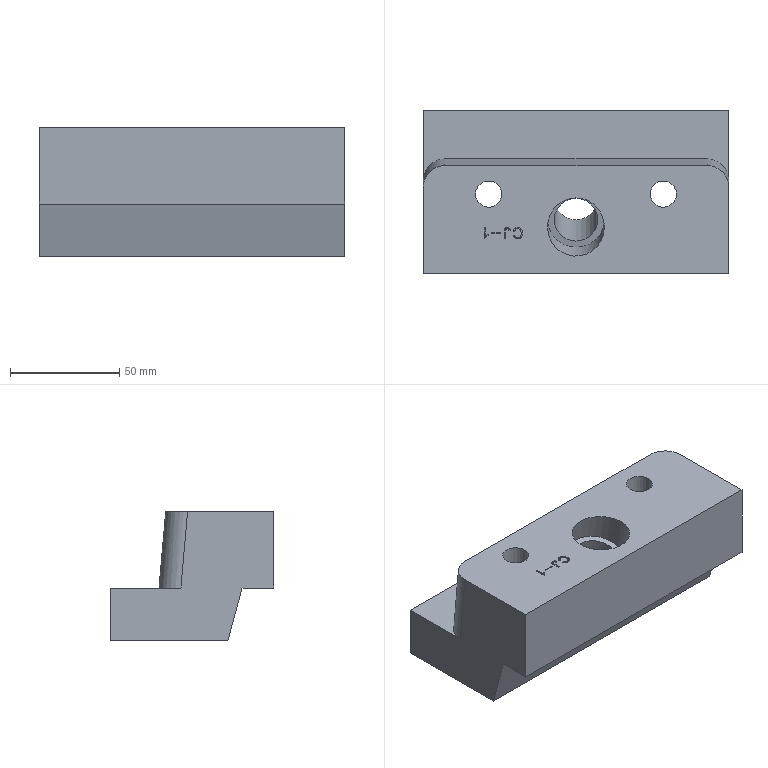Part | STEP file | solid 144 | 1 solid | 46 faces | box 140 x 75 x 59 mm | volume 401868 mm3 | plane 32 | cylinder 8 | other 6 | commonest cylinder face diameters 20 x3 12 x2 18 x2 26 x1